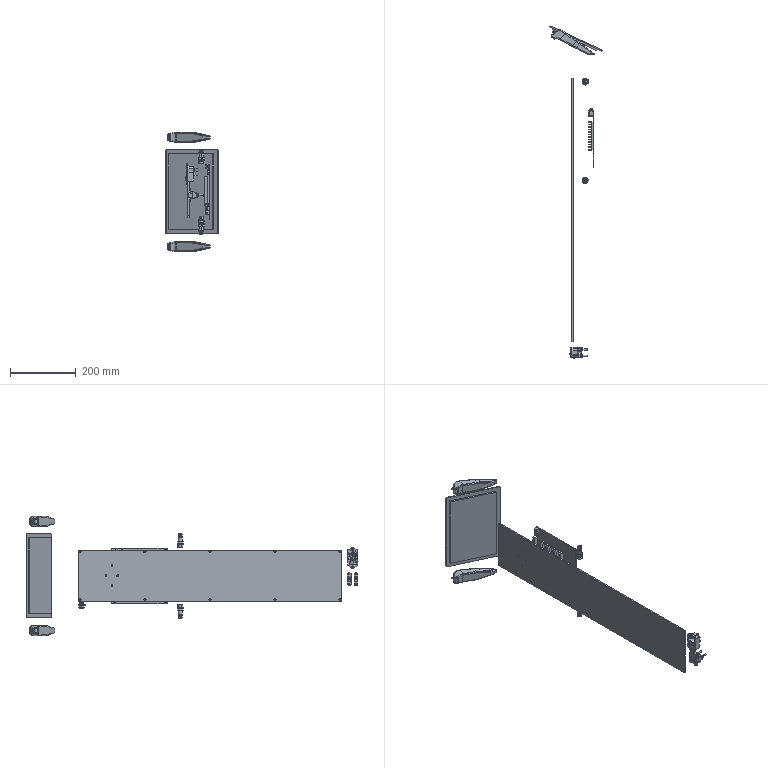Part | SolidWorks | features BaseBody 22, Fillet 2, ICE 2, Cut 1 | 20 solids | 1451 faces | box 159.207 x 1008 x 361.7 mm | volume 990994 mm3 | plane 811 | cylinder 373 | spline 135 | cone 60 | torus 46 | sphere 26 | commonest cylinder face diameters 1 x74 6 x36 4 x24 2.6 x22 3.4 x20 5 x20